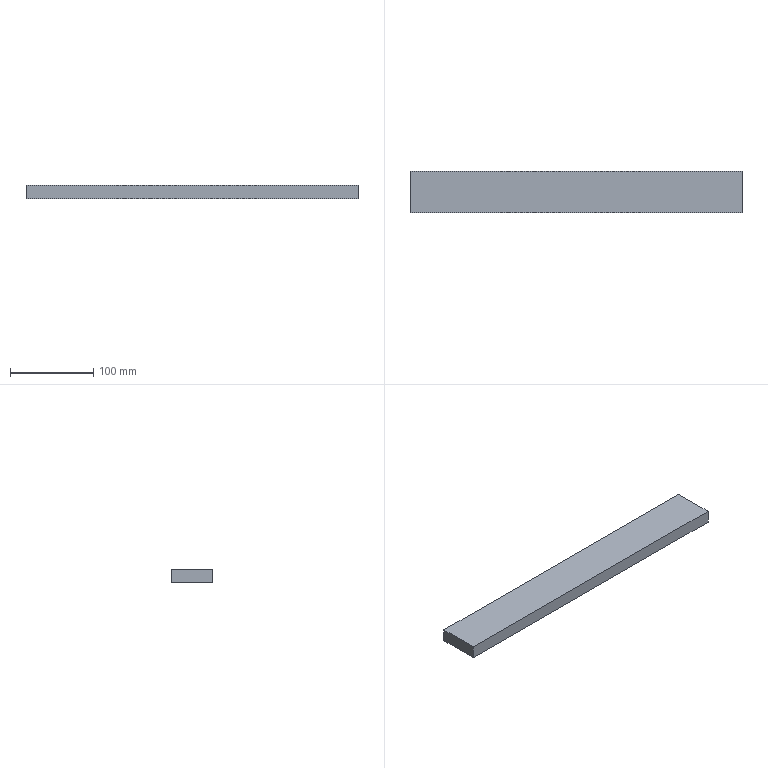Part | STEP file | 436_id790_x_t | 1 solid | 6 faces | box 400 x 50 x 16 mm | volume 320000 mm3 | plane 6
STEP:
#1=CARTESIAN_POINT('',(0.,0.,0.));
#2=DIRECTION('',(0.,0.,1.));
#3=DIRECTION('',(1.,0.,0.));
#4=AXIS2_PLACEMENT_3D('',#1,#2,#3);
#5=CARTESIAN_POINT('',(-483.5,632.5,81.));
#6=VERTEX_POINT('',#5);
#7=CARTESIAN_POINT('',(-883.5,632.5,81.));
#8=VERTEX_POINT('',#7);
#9=CARTESIAN_POINT('',(-683.5,632.5,81.));
#10=DIRECTION('',(-1.,0.,0.));
#11=VECTOR('',#10,1.);
#12=LINE('',#9,#11);
#13=CARTESIAN_POINT('',(-683.5,657.5,81.));
#14=DIRECTION('',(0.,0.,1.));
#15=DIRECTION('',(1.,0.,0.));
#16=AXIS2_PLACEMENT_3D('',#13,#14,#15);
#17=PLANE('',#16);
#18=CARTESIAN_POINT('',(0.,-25.));
#19=DIRECTION('',(-1.,0.));
#20=VECTOR('',#19,1.);
#21=LINE('',#18,#20);
#22=(GEOMETRIC_REPRESENTATION_CONTEXT(2)PARAMETRIC_REPRESENTATION_CONTEXT()REPRESENTATION_CONTEXT('',''));
#23=DEFINITIONAL_REPRESENTATION('',(#21),#22);
#24=PCURVE('',#17,#23);
#25=CARTESIAN_POINT('',(-683.5,632.5,65.));
#26=DIRECTION('',(0.,-1.,0.));
#27=DIRECTION('',(0.,0.,-1.));
#28=AXIS2_PLACEMENT_3D('',#25,#26,#27);
#29=PLANE('',#28);
#30=CARTESIAN_POINT('',(-16.,0.));
#31=DIRECTION('',(0.,-1.));
#32=VECTOR('',#31,1.);
#33=LINE('',#30,#32);
#34=(GEOMETRIC_REPRESENTATION_CONTEXT(2)PARAMETRIC_REPRESENTATION_CONTEXT()REPRESENTATION_CONTEXT('',''));
#35=DEFINITIONAL_REPRESENTATION('',(#33),#34);
#36=PCURVE('',#29,#35);
#37=SURFACE_CURVE('',#12,(#24,#36),.PCURVE_S1.);
#38=EDGE_CURVE('',#6,#8,#37,.T.);
#39=ORIENTED_EDGE('',*,*,#38,.F.);
#40=CARTESIAN_POINT('',(-483.5,682.5,81.));
#41=VERTEX_POINT('',#40);
#42=CARTESIAN_POINT('',(-483.5,657.5,81.));
#43=DIRECTION('',(0.,-1.,0.));
#44=VECTOR('',#43,1.);
#45=LINE('',#42,#44);
#46=CARTESIAN_POINT('',(200.,0.));
#47=DIRECTION('',(0.,-1.));
#48=VECTOR('',#47,1.);
#49=LINE('',#46,#48);
#50=(GEOMETRIC_REPRESENTATION_CONTEXT(2)PARAMETRIC_REPRESENTATION_CONTEXT()REPRESENTATION_CONTEXT('',''));
#51=DEFINITIONAL_REPRESENTATION('',(#49),#50);
#52=PCURVE('',#17,#51);
#53=CARTESIAN_POINT('',(-483.5,657.5,65.));
#54=DIRECTION('',(1.,0.,0.));
#55=DIRECTION('',(0.,0.,-1.));
#56=AXIS2_PLACEMENT_3D('',#53,#54,#55);
#57=PLANE('',#56);
#58=CARTESIAN_POINT('',(-16.,0.));
#59=DIRECTION('',(0.,-1.));
#60=VECTOR('',#59,1.);
#61=LINE('',#58,#60);
#62=(GEOMETRIC_REPRESENTATION_CONTEXT(2)PARAMETRIC_REPRESENTATION_CONTEXT()REPRESENTATION_CONTEXT('',''));
#63=DEFINITIONAL_REPRESENTATION('',(#61),#62);
#64=PCURVE('',#57,#63);
#65=SURFACE_CURVE('',#45,(#52,#64),.PCURVE_S1.);
#66=EDGE_CURVE('',#41,#6,#65,.T.);
#67=ORIENTED_EDGE('',*,*,#66,.F.);
#68=CARTESIAN_POINT('',(-883.5,682.5,81.));
#69=VERTEX_POINT('',#68);
#70=CARTESIAN_POINT('',(-683.5,682.5,81.));
#71=DIRECTION('',(1.,0.,0.));
#72=VECTOR('',#71,1.);
#73=LINE('',#70,#72);
#74=CARTESIAN_POINT('',(0.,25.));
#75=DIRECTION('',(1.,0.));
#76=VECTOR('',#75,1.);
#77=LINE('',#74,#76);
#78=(GEOMETRIC_REPRESENTATION_CONTEXT(2)PARAMETRIC_REPRESENTATION_CONTEXT()REPRESENTATION_CONTEXT('',''));
#79=DEFINITIONAL_REPRESENTATION('',(#77),#78);
#80=PCURVE('',#17,#79);
#81=CARTESIAN_POINT('',(-683.5,682.5,65.));
#82=DIRECTION('',(0.,1.,0.));
#83=DIRECTION('',(0.,0.,1.));
#84=AXIS2_PLACEMENT_3D('',#81,#82,#83);
#85=PLANE('',#84);
#86=CARTESIAN_POINT('',(16.,0.));
#87=DIRECTION('',(0.,1.));
#88=VECTOR('',#87,1.);
#89=LINE('',#86,#88);
#90=(GEOMETRIC_REPRESENTATION_CONTEXT(2)PARAMETRIC_REPRESENTATION_CONTEXT()REPRESENTATION_CONTEXT('',''));
#91=DEFINITIONAL_REPRESENTATION('',(#89),#90);
#92=PCURVE('',#85,#91);
#93=SURFACE_CURVE('',#73,(#80,#92),.PCURVE_S1.);
#94=EDGE_CURVE('',#69,#41,#93,.T.);
#95=ORIENTED_EDGE('',*,*,#94,.F.);
#96=CARTESIAN_POINT('',(-883.5,657.5,81.));
#97=DIRECTION('',(0.,1.,0.));
#98=VECTOR('',#97,1.);
#99=LINE('',#96,#98);
#100=CARTESIAN_POINT('',(-200.,0.));
#101=DIRECTION('',(0.,1.));
#102=VECTOR('',#101,1.);
#103=LINE('',#100,#102);
#104=(GEOMETRIC_REPRESENTATION_CONTEXT(2)PARAMETRIC_REPRESENTATION_CONTEXT()REPRESENTATION_CONTEXT('',''));
#105=DEFINITIONAL_REPRESENTATION('',(#103),#104);
#106=PCURVE('',#17,#105);
#107=CARTESIAN_POINT('',(-883.5,657.5,65.));
#108=DIRECTION('',(-1.,0.,0.));
#109=DIRECTION('',(0.,0.,1.));
#110=AXIS2_PLACEMENT_3D('',#107,#108,#109);
#111=PLANE('',#110);
#112=CARTESIAN_POINT('',(16.,0.));
#113=DIRECTION('',(0.,1.));
#114=VECTOR('',#113,1.);
#115=LINE('',#112,#114);
#116=(GEOMETRIC_REPRESENTATION_CONTEXT(2)PARAMETRIC_REPRESENTATION_CONTEXT()REPRESENTATION_CONTEXT('',''));
#117=DEFINITIONAL_REPRESENTATION('',(#115),#116);
#118=PCURVE('',#111,#117);
#119=SURFACE_CURVE('',#99,(#106,#118),.PCURVE_S1.);
#120=EDGE_CURVE('',#8,#69,#119,.T.);
#121=ORIENTED_EDGE('',*,*,#120,.F.);
#122=EDGE_LOOP('',(#39,#67,#95,#121));
#123=FACE_BOUND('',#122,.T.);
#124=ADVANCED_FACE('',(#123),#17,.T.);
#125=CARTESIAN_POINT('',(-483.5,632.5,65.));
#126=VERTEX_POINT('',#125);
#127=CARTESIAN_POINT('',(-483.5,632.5,65.));
#128=DIRECTION('',(0.,0.,1.));
#129=VECTOR('',#128,1.);
#130=LINE('',#127,#129);
#131=CARTESIAN_POINT('',(0.,200.));
#132=DIRECTION('',(-1.,0.));
#133=VECTOR('',#132,1.);
#134=LINE('',#131,#133);
#135=(GEOMETRIC_REPRESENTATION_CONTEXT(2)PARAMETRIC_REPRESENTATION_CONTEXT()REPRESENTATION_CONTEXT('',''));
#136=DEFINITIONAL_REPRESENTATION('',(#134),#135);
#137=PCURVE('',#29,#136);
#138=CARTESIAN_POINT('',(0.,-25.));
#139=DIRECTION('',(-1.,0.));
#140=VECTOR('',#139,1.);
#141=LINE('',#138,#140);
#142=(GEOMETRIC_REPRESENTATION_CONTEXT(2)PARAMETRIC_REPRESENTATION_CONTEXT()REPRESENTATION_CONTEXT('',''));
#143=DEFINITIONAL_REPRESENTATION('',(#141),#142);
#144=PCURVE('',#57,#143);
#145=SURFACE_CURVE('',#130,(#137,#144),.PCURVE_S1.);
#146=EDGE_CURVE('',#126,#6,#145,.T.);
#147=ORIENTED_EDGE('',*,*,#146,.T.);
#148=ORIENTED_EDGE('',*,*,#38,.T.);
#149=CARTESIAN_POINT('',(-883.5,632.5,65.));
#150=VERTEX_POINT('',#149);
#151=CARTESIAN_POINT('',(-883.5,632.5,65.));
#152=DIRECTION('',(0.,0.,1.));
#153=VECTOR('',#152,1.);
#154=LINE('',#151,#153);
#155=CARTESIAN_POINT('',(0.,-200.));
#156=DIRECTION('',(-1.,0.));
#157=VECTOR('',#156,1.);
#158=LINE('',#155,#157);
#159=(GEOMETRIC_REPRESENTATION_CONTEXT(2)PARAMETRIC_REPRESENTATION_CONTEXT()REPRESENTATION_CONTEXT('',''));
#160=DEFINITIONAL_REPRESENTATION('',(#158),#159);
#161=PCURVE('',#29,#160);
#162=CARTESIAN_POINT('',(0.,-25.));
#163=DIRECTION('',(1.,0.));
#164=VECTOR('',#163,1.);
#165=LINE('',#162,#164);
#166=(GEOMETRIC_REPRESENTATION_CONTEXT(2)PARAMETRIC_REPRESENTATION_CONTEXT()REPRESENTATION_CONTEXT('',''));
#167=DEFINITIONAL_REPRESENTATION('',(#165),#166);
#168=PCURVE('',#111,#167);
#169=SURFACE_CURVE('',#154,(#161,#168),.PCURVE_S1.);
#170=EDGE_CURVE('',#150,#8,#169,.T.);
#171=ORIENTED_EDGE('',*,*,#170,.F.);
#172=CARTESIAN_POINT('',(-683.5,632.5,65.));
#173=DIRECTION('',(1.,0.,0.));
#174=VECTOR('',#173,1.);
#175=LINE('',#172,#174);
#176=CARTESIAN_POINT('',(0.,0.));
#177=DIRECTION('',(0.,1.));
#178=VECTOR('',#177,1.);
#179=LINE('',#176,#178);
#180=(GEOMETRIC_REPRESENTATION_CONTEXT(2)PARAMETRIC_REPRESENTATION_CONTEXT()REPRESENTATION_CONTEXT('',''));
#181=DEFINITIONAL_REPRESENTATION('',(#179),#180);
#182=PCURVE('',#29,#181);
#183=CARTESIAN_POINT('',(-683.5,657.5,65.));
#184=DIRECTION('',(0.,0.,-1.));
#185=DIRECTION('',(-1.,0.,0.));
#186=AXIS2_PLACEMENT_3D('',#183,#184,#185);
#187=PLANE('',#186);
#188=CARTESIAN_POINT('',(0.,-25.));
#189=DIRECTION('',(-1.,0.));
#190=VECTOR('',#189,1.);
#191=LINE('',#188,#190);
#192=(GEOMETRIC_REPRESENTATION_CONTEXT(2)PARAMETRIC_REPRESENTATION_CONTEXT()REPRESENTATION_CONTEXT('',''));
#193=DEFINITIONAL_REPRESENTATION('',(#191),#192);
#194=PCURVE('',#187,#193);
#195=SURFACE_CURVE('',#175,(#182,#194),.PCURVE_S1.);
#196=EDGE_CURVE('',#150,#126,#195,.T.);
#197=ORIENTED_EDGE('',*,*,#196,.T.);
#198=EDGE_LOOP('',(#147,#148,#171,#197));
#199=FACE_BOUND('',#198,.T.);
#200=ADVANCED_FACE('',(#199),#29,.T.);
#201=ORIENTED_EDGE('',*,*,#170,.T.);
#202=ORIENTED_EDGE('',*,*,#120,.T.);
#203=CARTESIAN_POINT('',(-883.5,682.5,65.));
#204=VERTEX_POINT('',#203);
#205=CARTESIAN_POINT('',(-883.5,682.5,65.));
#206=DIRECTION('',(0.,0.,1.));
#207=VECTOR('',#206,1.);
#208=LINE('',#205,#207);
#209=CARTESIAN_POINT('',(0.,25.));
#210=DIRECTION('',(1.,0.));
#211=VECTOR('',#210,1.);
#212=LINE('',#209,#211);
#213=(GEOMETRIC_REPRESENTATION_CONTEXT(2)PARAMETRIC_REPRESENTATION_CONTEXT()REPRESENTATION_CONTEXT('',''));
#214=DEFINITIONAL_REPRESENTATION('',(#212),#213);
#215=PCURVE('',#111,#214);
#216=CARTESIAN_POINT('',(0.,-200.));
#217=DIRECTION('',(1.,0.));
#218=VECTOR('',#217,1.);
#219=LINE('',#216,#218);
#220=(GEOMETRIC_REPRESENTATION_CONTEXT(2)PARAMETRIC_REPRESENTATION_CONTEXT()REPRESENTATION_CONTEXT('',''));
#221=DEFINITIONAL_REPRESENTATION('',(#219),#220);
#222=PCURVE('',#85,#221);
#223=SURFACE_CURVE('',#208,(#215,#222),.PCURVE_S1.);
#224=EDGE_CURVE('',#204,#69,#223,.T.);
#225=ORIENTED_EDGE('',*,*,#224,.F.);
#226=CARTESIAN_POINT('',(-883.5,657.5,65.));
#227=DIRECTION('',(0.,-1.,0.));
#228=VECTOR('',#227,1.);
#229=LINE('',#226,#228);
#230=CARTESIAN_POINT('',(0.,0.));
#231=DIRECTION('',(0.,-1.));
#232=VECTOR('',#231,1.);
#233=LINE('',#230,#232);
#234=(GEOMETRIC_REPRESENTATION_CONTEXT(2)PARAMETRIC_REPRESENTATION_CONTEXT()REPRESENTATION_CONTEXT('',''));
#235=DEFINITIONAL_REPRESENTATION('',(#233),#234);
#236=PCURVE('',#111,#235);
#237=CARTESIAN_POINT('',(200.,0.));
#238=DIRECTION('',(0.,-1.));
#239=VECTOR('',#238,1.);
#240=LINE('',#237,#239);
#241=(GEOMETRIC_REPRESENTATION_CONTEXT(2)PARAMETRIC_REPRESENTATION_CONTEXT()REPRESENTATION_CONTEXT('',''));
#242=DEFINITIONAL_REPRESENTATION('',(#240),#241);
#243=PCURVE('',#187,#242);
#244=SURFACE_CURVE('',#229,(#236,#243),.PCURVE_S1.);
#245=EDGE_CURVE('',#204,#150,#244,.T.);
#246=ORIENTED_EDGE('',*,*,#245,.T.);
#247=EDGE_LOOP('',(#201,#202,#225,#246));
#248=FACE_BOUND('',#247,.T.);
#249=ADVANCED_FACE('',(#248),#111,.T.);
#250=ORIENTED_EDGE('',*,*,#224,.T.);
#251=ORIENTED_EDGE('',*,*,#94,.T.);
#252=CARTESIAN_POINT('',(-483.5,682.5,65.));
#253=VERTEX_POINT('',#252);
#254=CARTESIAN_POINT('',(-483.5,682.5,65.));
#255=DIRECTION('',(0.,0.,1.));
#256=VECTOR('',#255,1.);
#257=LINE('',#254,#256);
#258=CARTESIAN_POINT('',(0.,200.));
#259=DIRECTION('',(1.,0.));
#260=VECTOR('',#259,1.);
#261=LINE('',#258,#260);
#262=(GEOMETRIC_REPRESENTATION_CONTEXT(2)PARAMETRIC_REPRESENTATION_CONTEXT()REPRESENTATION_CONTEXT('',''));
#263=DEFINITIONAL_REPRESENTATION('',(#261),#262);
#264=PCURVE('',#85,#263);
#265=CARTESIAN_POINT('',(0.,25.));
#266=DIRECTION('',(-1.,0.));
#267=VECTOR('',#266,1.);
#268=LINE('',#265,#267);
#269=(GEOMETRIC_REPRESENTATION_CONTEXT(2)PARAMETRIC_REPRESENTATION_CONTEXT()REPRESENTATION_CONTEXT('',''));
#270=DEFINITIONAL_REPRESENTATION('',(#268),#269);
#271=PCURVE('',#57,#270);
#272=SURFACE_CURVE('',#257,(#264,#271),.PCURVE_S1.);
#273=EDGE_CURVE('',#253,#41,#272,.T.);
#274=ORIENTED_EDGE('',*,*,#273,.F.);
#275=CARTESIAN_POINT('',(-683.5,682.5,65.));
#276=DIRECTION('',(-1.,0.,0.));
#277=VECTOR('',#276,1.);
#278=LINE('',#275,#277);
#279=CARTESIAN_POINT('',(0.,0.));
#280=DIRECTION('',(0.,-1.));
#281=VECTOR('',#280,1.);
#282=LINE('',#279,#281);
#283=(GEOMETRIC_REPRESENTATION_CONTEXT(2)PARAMETRIC_REPRESENTATION_CONTEXT()REPRESENTATION_CONTEXT('',''));
#284=DEFINITIONAL_REPRESENTATION('',(#282),#283);
#285=PCURVE('',#85,#284);
#286=CARTESIAN_POINT('',(0.,25.));
#287=DIRECTION('',(1.,0.));
#288=VECTOR('',#287,1.);
#289=LINE('',#286,#288);
#290=(GEOMETRIC_REPRESENTATION_CONTEXT(2)PARAMETRIC_REPRESENTATION_CONTEXT()REPRESENTATION_CONTEXT('',''));
#291=DEFINITIONAL_REPRESENTATION('',(#289),#290);
#292=PCURVE('',#187,#291);
#293=SURFACE_CURVE('',#278,(#285,#292),.PCURVE_S1.);
#294=EDGE_CURVE('',#253,#204,#293,.T.);
#295=ORIENTED_EDGE('',*,*,#294,.T.);
#296=EDGE_LOOP('',(#250,#251,#274,#295));
#297=FACE_BOUND('',#296,.T.);
#298=ADVANCED_FACE('',(#297),#85,.T.);
#299=CARTESIAN_POINT('',(-483.5,657.5,65.));
#300=DIRECTION('',(0.,1.,0.));
#301=VECTOR('',#300,1.);
#302=LINE('',#299,#301);
#303=CARTESIAN_POINT('',(-200.,0.));
#304=DIRECTION('',(0.,1.));
#305=VECTOR('',#304,1.);
#306=LINE('',#303,#305);
#307=(GEOMETRIC_REPRESENTATION_CONTEXT(2)PARAMETRIC_REPRESENTATION_CONTEXT()REPRESENTATION_CONTEXT('',''));
#308=DEFINITIONAL_REPRESENTATION('',(#306),#307);
#309=PCURVE('',#187,#308);
#310=CARTESIAN_POINT('',(0.,0.));
#311=DIRECTION('',(0.,1.));
#312=VECTOR('',#311,1.);
#313=LINE('',#310,#312);
#314=(GEOMETRIC_REPRESENTATION_CONTEXT(2)PARAMETRIC_REPRESENTATION_CONTEXT()REPRESENTATION_CONTEXT('',''));
#315=DEFINITIONAL_REPRESENTATION('',(#313),#314);
#316=PCURVE('',#57,#315);
#317=SURFACE_CURVE('',#302,(#309,#316),.PCURVE_S1.);
#318=EDGE_CURVE('',#126,#253,#317,.T.);
#319=ORIENTED_EDGE('',*,*,#318,.F.);
#320=ORIENTED_EDGE('',*,*,#196,.F.);
#321=ORIENTED_EDGE('',*,*,#245,.F.);
#322=ORIENTED_EDGE('',*,*,#294,.F.);
#323=EDGE_LOOP('',(#319,#320,#321,#322));
#324=FACE_BOUND('',#323,.T.);
#325=ADVANCED_FACE('',(#324),#187,.T.);
#326=ORIENTED_EDGE('',*,*,#318,.T.);
#327=ORIENTED_EDGE('',*,*,#273,.T.);
#328=ORIENTED_EDGE('',*,*,#66,.T.);
#329=ORIENTED_EDGE('',*,*,#146,.F.);
#330=EDGE_LOOP('',(#326,#327,#328,#329));
#331=FACE_BOUND('',#330,.T.);
#332=ADVANCED_FACE('',(#331),#57,.T.);
#333=CLOSED_SHELL('',(#124,#200,#249,#298,#325,#332));
#334=MANIFOLD_SOLID_BREP('',#333);
#335=(LENGTH_UNIT()NAMED_UNIT(*)SI_UNIT(.MILLI.,.METRE.));
#336=UNCERTAINTY_MEASURE_WITH_UNIT(LENGTH_MEASURE(0.0000001),#335,'','');
#337=(NAMED_UNIT(*)PLANE_ANGLE_UNIT()SI_UNIT($,.RADIAN.));
#338=(NAMED_UNIT(*)SI_UNIT($,.STERADIAN.)SOLID_ANGLE_UNIT());
#339=(GEOMETRIC_REPRESENTATION_CONTEXT(3)GLOBAL_UNCERTAINTY_ASSIGNED_CONTEXT((#336))GLOBAL_UNIT_ASSIGNED_CONTEXT((#335,#337,#338))REPRESENTATION_CONTEXT('',''));
#340=ADVANCED_BREP_SHAPE_REPRESENTATION('',(#4,#334),#339);